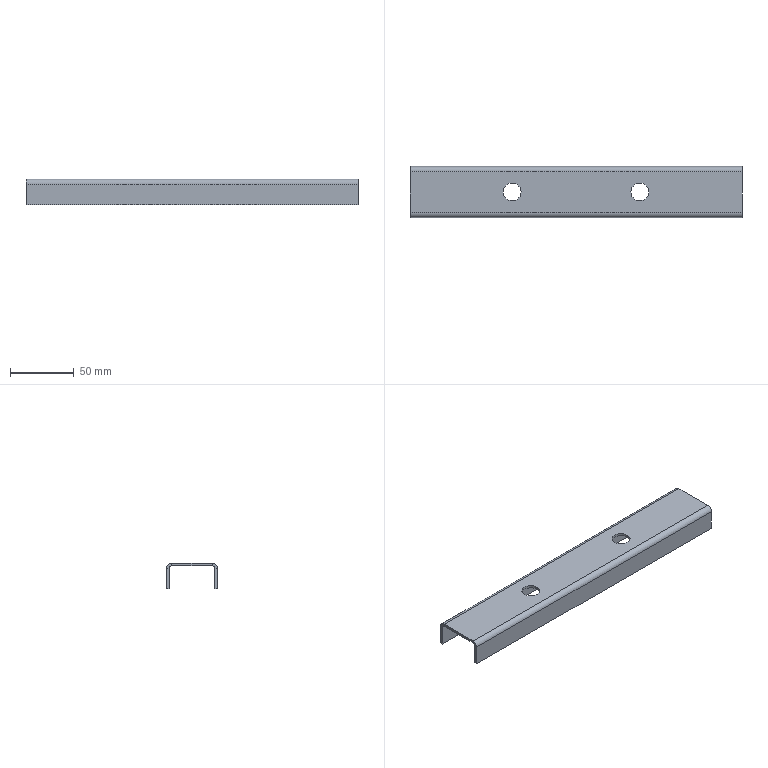Part | STEP file | Produce dryer line heating fan-OVEN-454 | 1 solid | 26 faces | box 260 x 40 x 20 mm | volume 37565 mm3 | plane 18 | cylinder 8 | commonest cylinder face diameters 14 x4 4 x2 8 x2
STEP:
#1=CARTESIAN_POINT('',(57.,20.,-2.));
#2=VERTEX_POINT('',#1);
#3=CARTESIAN_POINT('',(43.,20.,-2.));
#4=VERTEX_POINT('',#3);
#5=CARTESIAN_POINT('',(50.,20.,-2.));
#6=DIRECTION('',(0.,0.,-1.));
#7=DIRECTION('',(-1.,0.,0.));
#8=AXIS2_PLACEMENT_3D('',#5,#6,#7);
#9=CIRCLE('',#8,7.);
#10=EDGE_CURVE('',#2,#4,#9,.T.);
#11=ORIENTED_EDGE('',*,*,#10,.T.);
#12=CARTESIAN_POINT('',(43.,20.,0.));
#13=VERTEX_POINT('',#12);
#14=CARTESIAN_POINT('',(43.,20.,-10.));
#15=DIRECTION('',(0.,0.,1.));
#16=VECTOR('',#15,1000.);
#17=LINE('',#14,#16);
#18=EDGE_CURVE('',#4,#13,#17,.T.);
#19=ORIENTED_EDGE('',*,*,#18,.T.);
#20=CARTESIAN_POINT('',(57.,20.,0.));
#21=VERTEX_POINT('',#20);
#22=CARTESIAN_POINT('',(50.,20.,0.));
#23=DIRECTION('',(0.,0.,1.));
#24=DIRECTION('',(1.,0.,0.));
#25=AXIS2_PLACEMENT_3D('',#22,#23,#24);
#26=CIRCLE('',#25,7.);
#27=EDGE_CURVE('',#13,#21,#26,.T.);
#28=ORIENTED_EDGE('',*,*,#27,.T.);
#29=CARTESIAN_POINT('',(57.,20.,-10.));
#30=DIRECTION('',(0.,0.,1.));
#31=VECTOR('',#30,1000.);
#32=LINE('',#29,#31);
#33=EDGE_CURVE('',#2,#21,#32,.T.);
#34=ORIENTED_EDGE('',*,*,#33,.F.);
#35=EDGE_LOOP('',(#11,#19,#28,#34));
#36=FACE_OUTER_BOUND('',#35,.T.);
#37=CARTESIAN_POINT('',(50.,20.,-10.));
#38=DIRECTION('',(0.,0.,1.));
#39=DIRECTION('',(1.,0.,0.));
#40=AXIS2_PLACEMENT_3D('',#37,#38,#39);
#41=CYLINDRICAL_SURFACE('',#40,7.);
#42=ADVANCED_FACE('',(#36),#41,.F.);
#43=CARTESIAN_POINT('',(-43.,20.,-2.));
#44=VERTEX_POINT('',#43);
#45=CARTESIAN_POINT('',(-57.,20.,-2.));
#46=VERTEX_POINT('',#45);
#47=CARTESIAN_POINT('',(-50.,20.,-2.));
#48=DIRECTION('',(0.,0.,-1.));
#49=DIRECTION('',(-1.,0.,0.));
#50=AXIS2_PLACEMENT_3D('',#47,#48,#49);
#51=CIRCLE('',#50,7.);
#52=EDGE_CURVE('',#44,#46,#51,.T.);
#53=ORIENTED_EDGE('',*,*,#52,.T.);
#54=CARTESIAN_POINT('',(-57.,20.,0.));
#55=VERTEX_POINT('',#54);
#56=CARTESIAN_POINT('',(-57.,20.,-10.));
#57=DIRECTION('',(0.,0.,1.));
#58=VECTOR('',#57,1000.);
#59=LINE('',#56,#58);
#60=EDGE_CURVE('',#46,#55,#59,.T.);
#61=ORIENTED_EDGE('',*,*,#60,.T.);
#62=CARTESIAN_POINT('',(-43.,20.,0.));
#63=VERTEX_POINT('',#62);
#64=CARTESIAN_POINT('',(-50.,20.,0.));
#65=DIRECTION('',(0.,0.,1.));
#66=DIRECTION('',(1.,0.,0.));
#67=AXIS2_PLACEMENT_3D('',#64,#65,#66);
#68=CIRCLE('',#67,7.);
#69=EDGE_CURVE('',#55,#63,#68,.T.);
#70=ORIENTED_EDGE('',*,*,#69,.T.);
#71=CARTESIAN_POINT('',(-43.,20.,-10.));
#72=DIRECTION('',(0.,0.,1.));
#73=VECTOR('',#72,1000.);
#74=LINE('',#71,#73);
#75=EDGE_CURVE('',#44,#63,#74,.T.);
#76=ORIENTED_EDGE('',*,*,#75,.F.);
#77=EDGE_LOOP('',(#53,#61,#70,#76));
#78=FACE_OUTER_BOUND('',#77,.T.);
#79=CARTESIAN_POINT('',(-50.,20.,-10.));
#80=DIRECTION('',(0.,0.,1.));
#81=DIRECTION('',(1.,0.,0.));
#82=AXIS2_PLACEMENT_3D('',#79,#80,#81);
#83=CYLINDRICAL_SURFACE('',#82,7.);
#84=ADVANCED_FACE('',(#78),#83,.F.);
#85=CARTESIAN_POINT('',(130.,4.,0.));
#86=VERTEX_POINT('',#85);
#87=CARTESIAN_POINT('',(130.,4.,-2.));
#88=VERTEX_POINT('',#87);
#89=CARTESIAN_POINT('',(130.,4.,0.));
#90=DIRECTION('',(0.,0.,-1.));
#91=VECTOR('',#90,1000.);
#92=LINE('',#89,#91);
#93=EDGE_CURVE('',#86,#88,#92,.T.);
#94=ORIENTED_EDGE('',*,*,#93,.F.);
#95=CARTESIAN_POINT('',(130.,0.,-4.));
#96=VERTEX_POINT('',#95);
#97=CARTESIAN_POINT('',(130.,4.,-4.));
#98=DIRECTION('',(1.,0.,0.));
#99=DIRECTION('',(0.,0.,-1.));
#100=AXIS2_PLACEMENT_3D('',#97,#98,#99);
#101=CIRCLE('',#100,4.);
#102=EDGE_CURVE('',#86,#96,#101,.T.);
#103=ORIENTED_EDGE('',*,*,#102,.T.);
#104=CARTESIAN_POINT('',(130.,2.,-4.));
#105=VERTEX_POINT('',#104);
#106=CARTESIAN_POINT('',(130.,2.,-4.));
#107=DIRECTION('',(0.,-1.,0.));
#108=VECTOR('',#107,1000.);
#109=LINE('',#106,#108);
#110=EDGE_CURVE('',#105,#96,#109,.T.);
#111=ORIENTED_EDGE('',*,*,#110,.F.);
#112=CARTESIAN_POINT('',(130.,4.,-4.));
#113=DIRECTION('',(1.,0.,0.));
#114=DIRECTION('',(0.,0.,-1.));
#115=AXIS2_PLACEMENT_3D('',#112,#113,#114);
#116=CIRCLE('',#115,2.);
#117=EDGE_CURVE('',#88,#105,#116,.T.);
#118=ORIENTED_EDGE('',*,*,#117,.F.);
#119=EDGE_LOOP('',(#94,#103,#111,#118));
#120=FACE_OUTER_BOUND('',#119,.T.);
#121=CARTESIAN_POINT('',(130.,4.,0.));
#122=DIRECTION('',(1.,0.,0.));
#123=DIRECTION('',(0.,0.,-1.));
#124=AXIS2_PLACEMENT_3D('',#121,#122,#123);
#125=PLANE('',#124);
#126=ADVANCED_FACE('',(#120),#125,.T.);
#127=CARTESIAN_POINT('',(130.,36.,0.));
#128=VERTEX_POINT('',#127);
#129=CARTESIAN_POINT('',(130.,40.,0.));
#130=DIRECTION('',(0.,-1.,0.));
#131=VECTOR('',#130,1000.);
#132=LINE('',#129,#131);
#133=EDGE_CURVE('',#128,#86,#132,.T.);
#134=ORIENTED_EDGE('',*,*,#133,.T.);
#135=ORIENTED_EDGE('',*,*,#93,.T.);
#136=CARTESIAN_POINT('',(130.,36.,-2.));
#137=VERTEX_POINT('',#136);
#138=CARTESIAN_POINT('',(130.,40.,-2.));
#139=DIRECTION('',(0.,-1.,0.));
#140=VECTOR('',#139,1000.);
#141=LINE('',#138,#140);
#142=EDGE_CURVE('',#137,#88,#141,.T.);
#143=ORIENTED_EDGE('',*,*,#142,.F.);
#144=CARTESIAN_POINT('',(130.,36.,-2.));
#145=DIRECTION('',(0.,0.,1.));
#146=VECTOR('',#145,1000.);
#147=LINE('',#144,#146);
#148=EDGE_CURVE('',#137,#128,#147,.T.);
#149=ORIENTED_EDGE('',*,*,#148,.T.);
#150=EDGE_LOOP('',(#134,#135,#143,#149));
#151=FACE_OUTER_BOUND('',#150,.T.);
#152=CARTESIAN_POINT('',(130.,2.,-4.));
#153=DIRECTION('',(1.,0.,0.));
#154=DIRECTION('',(0.,0.,-1.));
#155=AXIS2_PLACEMENT_3D('',#152,#153,#154);
#156=PLANE('',#155);
#157=ADVANCED_FACE('',(#151),#156,.T.);
#158=CARTESIAN_POINT('',(-130.,0.,-4.));
#159=VERTEX_POINT('',#158);
#160=CARTESIAN_POINT('',(-130.,2.,-4.));
#161=VERTEX_POINT('',#160);
#162=CARTESIAN_POINT('',(-130.,0.,-4.));
#163=DIRECTION('',(0.,1.,0.));
#164=VECTOR('',#163,1000.);
#165=LINE('',#162,#164);
#166=EDGE_CURVE('',#159,#161,#165,.T.);
#167=ORIENTED_EDGE('',*,*,#166,.F.);
#168=CARTESIAN_POINT('',(-130.,4.,0.));
#169=VERTEX_POINT('',#168);
#170=CARTESIAN_POINT('',(-130.,4.,-4.));
#171=DIRECTION('',(1.,0.,0.));
#172=DIRECTION('',(0.,0.,-1.));
#173=AXIS2_PLACEMENT_3D('',#170,#171,#172);
#174=CIRCLE('',#173,4.);
#175=EDGE_CURVE('',#169,#159,#174,.T.);
#176=ORIENTED_EDGE('',*,*,#175,.F.);
#177=CARTESIAN_POINT('',(-130.,4.,-2.));
#178=VERTEX_POINT('',#177);
#179=CARTESIAN_POINT('',(-130.,4.,-2.));
#180=DIRECTION('',(0.,0.,1.));
#181=VECTOR('',#180,1000.);
#182=LINE('',#179,#181);
#183=EDGE_CURVE('',#178,#169,#182,.T.);
#184=ORIENTED_EDGE('',*,*,#183,.F.);
#185=CARTESIAN_POINT('',(-130.,4.,-4.));
#186=DIRECTION('',(1.,0.,0.));
#187=DIRECTION('',(0.,0.,-1.));
#188=AXIS2_PLACEMENT_3D('',#185,#186,#187);
#189=CIRCLE('',#188,2.);
#190=EDGE_CURVE('',#178,#161,#189,.T.);
#191=ORIENTED_EDGE('',*,*,#190,.T.);
#192=EDGE_LOOP('',(#167,#176,#184,#191));
#193=FACE_OUTER_BOUND('',#192,.T.);
#194=CARTESIAN_POINT('',(-130.,0.,-4.));
#195=DIRECTION('',(-1.,0.,0.));
#196=DIRECTION('',(0.,0.,1.));
#197=AXIS2_PLACEMENT_3D('',#194,#195,#196);
#198=PLANE('',#197);
#199=ADVANCED_FACE('',(#193),#198,.T.);
#200=CARTESIAN_POINT('',(-130.,0.,-20.));
#201=VERTEX_POINT('',#200);
#202=CARTESIAN_POINT('',(-130.,0.,0.));
#203=DIRECTION('',(0.,0.,-1.));
#204=VECTOR('',#203,1000.);
#205=LINE('',#202,#204);
#206=EDGE_CURVE('',#159,#201,#205,.T.);
#207=ORIENTED_EDGE('',*,*,#206,.F.);
#208=ORIENTED_EDGE('',*,*,#166,.T.);
#209=CARTESIAN_POINT('',(-130.,2.,-20.));
#210=VERTEX_POINT('',#209);
#211=CARTESIAN_POINT('',(-130.,2.,0.));
#212=DIRECTION('',(0.,0.,-1.));
#213=VECTOR('',#212,1000.);
#214=LINE('',#211,#213);
#215=EDGE_CURVE('',#161,#210,#214,.T.);
#216=ORIENTED_EDGE('',*,*,#215,.T.);
#217=CARTESIAN_POINT('',(-130.,2.,-20.));
#218=DIRECTION('',(0.,-1.,0.));
#219=VECTOR('',#218,1000.);
#220=LINE('',#217,#219);
#221=EDGE_CURVE('',#210,#201,#220,.T.);
#222=ORIENTED_EDGE('',*,*,#221,.T.);
#223=EDGE_LOOP('',(#207,#208,#216,#222));
#224=FACE_OUTER_BOUND('',#223,.T.);
#225=CARTESIAN_POINT('',(-130.,4.,-2.));
#226=DIRECTION('',(-1.,0.,0.));
#227=DIRECTION('',(0.,0.,1.));
#228=AXIS2_PLACEMENT_3D('',#225,#226,#227);
#229=PLANE('',#228);
#230=ADVANCED_FACE('',(#224),#229,.T.);
#231=CARTESIAN_POINT('',(130.,40.,-4.));
#232=VERTEX_POINT('',#231);
#233=CARTESIAN_POINT('',(130.,38.,-4.));
#234=VERTEX_POINT('',#233);
#235=CARTESIAN_POINT('',(130.,40.,-4.));
#236=DIRECTION('',(0.,-1.,0.));
#237=VECTOR('',#236,1000.);
#238=LINE('',#235,#237);
#239=EDGE_CURVE('',#232,#234,#238,.T.);
#240=ORIENTED_EDGE('',*,*,#239,.F.);
#241=CARTESIAN_POINT('',(130.,36.,-4.));
#242=DIRECTION('',(1.,0.,0.));
#243=DIRECTION('',(0.,0.,-1.));
#244=AXIS2_PLACEMENT_3D('',#241,#242,#243);
#245=CIRCLE('',#244,4.);
#246=EDGE_CURVE('',#232,#128,#245,.T.);
#247=ORIENTED_EDGE('',*,*,#246,.T.);
#248=ORIENTED_EDGE('',*,*,#148,.F.);
#249=CARTESIAN_POINT('',(130.,36.,-4.));
#250=DIRECTION('',(1.,0.,0.));
#251=DIRECTION('',(0.,0.,-1.));
#252=AXIS2_PLACEMENT_3D('',#249,#250,#251);
#253=CIRCLE('',#252,2.);
#254=EDGE_CURVE('',#234,#137,#253,.T.);
#255=ORIENTED_EDGE('',*,*,#254,.F.);
#256=EDGE_LOOP('',(#240,#247,#248,#255));
#257=FACE_OUTER_BOUND('',#256,.T.);
#258=CARTESIAN_POINT('',(130.,40.,-4.));
#259=DIRECTION('',(1.,0.,0.));
#260=DIRECTION('',(0.,0.,-1.));
#261=AXIS2_PLACEMENT_3D('',#258,#259,#260);
#262=PLANE('',#261);
#263=ADVANCED_FACE('',(#257),#262,.T.);
#264=CARTESIAN_POINT('',(130.,40.,-20.));
#265=VERTEX_POINT('',#264);
#266=CARTESIAN_POINT('',(130.,40.,0.));
#267=DIRECTION('',(0.,0.,1.));
#268=VECTOR('',#267,1000.);
#269=LINE('',#266,#268);
#270=EDGE_CURVE('',#265,#232,#269,.T.);
#271=ORIENTED_EDGE('',*,*,#270,.T.);
#272=ORIENTED_EDGE('',*,*,#239,.T.);
#273=CARTESIAN_POINT('',(130.,38.,-20.));
#274=VERTEX_POINT('',#273);
#275=CARTESIAN_POINT('',(130.,38.,0.));
#276=DIRECTION('',(0.,0.,1.));
#277=VECTOR('',#276,1000.);
#278=LINE('',#275,#277);
#279=EDGE_CURVE('',#274,#234,#278,.T.);
#280=ORIENTED_EDGE('',*,*,#279,.F.);
#281=CARTESIAN_POINT('',(130.,40.,-20.));
#282=DIRECTION('',(0.,-1.,0.));
#283=VECTOR('',#282,1000.);
#284=LINE('',#281,#283);
#285=EDGE_CURVE('',#265,#274,#284,.T.);
#286=ORIENTED_EDGE('',*,*,#285,.F.);
#287=EDGE_LOOP('',(#271,#272,#280,#286));
#288=FACE_OUTER_BOUND('',#287,.T.);
#289=CARTESIAN_POINT('',(130.,36.,-2.));
#290=DIRECTION('',(1.,0.,0.));
#291=DIRECTION('',(0.,0.,-1.));
#292=AXIS2_PLACEMENT_3D('',#289,#290,#291);
#293=PLANE('',#292);
#294=ADVANCED_FACE('',(#288),#293,.T.);
#295=CARTESIAN_POINT('',(-130.,36.,0.));
#296=VERTEX_POINT('',#295);
#297=CARTESIAN_POINT('',(-130.,36.,-2.));
#298=VERTEX_POINT('',#297);
#299=CARTESIAN_POINT('',(-130.,36.,0.));
#300=DIRECTION('',(0.,0.,-1.));
#301=VECTOR('',#300,1000.);
#302=LINE('',#299,#301);
#303=EDGE_CURVE('',#296,#298,#302,.T.);
#304=ORIENTED_EDGE('',*,*,#303,.F.);
#305=CARTESIAN_POINT('',(-130.,40.,-4.));
#306=VERTEX_POINT('',#305);
#307=CARTESIAN_POINT('',(-130.,36.,-4.));
#308=DIRECTION('',(1.,0.,0.));
#309=DIRECTION('',(0.,0.,-1.));
#310=AXIS2_PLACEMENT_3D('',#307,#308,#309);
#311=CIRCLE('',#310,4.);
#312=EDGE_CURVE('',#306,#296,#311,.T.);
#313=ORIENTED_EDGE('',*,*,#312,.F.);
#314=CARTESIAN_POINT('',(-130.,38.,-4.));
#315=VERTEX_POINT('',#314);
#316=CARTESIAN_POINT('',(-130.,38.,-4.));
#317=DIRECTION('',(0.,1.,0.));
#318=VECTOR('',#317,1000.);
#319=LINE('',#316,#318);
#320=EDGE_CURVE('',#315,#306,#319,.T.);
#321=ORIENTED_EDGE('',*,*,#320,.F.);
#322=CARTESIAN_POINT('',(-130.,36.,-4.));
#323=DIRECTION('',(1.,0.,0.));
#324=DIRECTION('',(0.,0.,-1.));
#325=AXIS2_PLACEMENT_3D('',#322,#323,#324);
#326=CIRCLE('',#325,2.);
#327=EDGE_CURVE('',#315,#298,#326,.T.);
#328=ORIENTED_EDGE('',*,*,#327,.T.);
#329=EDGE_LOOP('',(#304,#313,#321,#328));
#330=FACE_OUTER_BOUND('',#329,.T.);
#331=CARTESIAN_POINT('',(-130.,36.,0.));
#332=DIRECTION('',(-1.,0.,0.));
#333=DIRECTION('',(0.,0.,1.));
#334=AXIS2_PLACEMENT_3D('',#331,#332,#333);
#335=PLANE('',#334);
#336=ADVANCED_FACE('',(#330),#335,.T.);
#337=CARTESIAN_POINT('',(-130.,40.,0.));
#338=DIRECTION('',(0.,-1.,0.));
#339=VECTOR('',#338,1000.);
#340=LINE('',#337,#339);
#341=EDGE_CURVE('',#296,#169,#340,.T.);
#342=ORIENTED_EDGE('',*,*,#341,.F.);
#343=ORIENTED_EDGE('',*,*,#303,.T.);
#344=CARTESIAN_POINT('',(-130.,40.,-2.));
#345=DIRECTION('',(0.,-1.,0.));
#346=VECTOR('',#345,1000.);
#347=LINE('',#344,#346);
#348=EDGE_CURVE('',#298,#178,#347,.T.);
#349=ORIENTED_EDGE('',*,*,#348,.T.);
#350=ORIENTED_EDGE('',*,*,#183,.T.);
#351=EDGE_LOOP('',(#342,#343,#349,#350));
#352=FACE_OUTER_BOUND('',#351,.T.);
#353=CARTESIAN_POINT('',(-130.,38.,-4.));
#354=DIRECTION('',(-1.,0.,0.));
#355=DIRECTION('',(0.,0.,1.));
#356=AXIS2_PLACEMENT_3D('',#353,#354,#355);
#357=PLANE('',#356);
#358=ADVANCED_FACE('',(#352),#357,.T.);
#359=ORIENTED_EDGE('',*,*,#206,.T.);
#360=CARTESIAN_POINT('',(130.,0.,-20.));
#361=VERTEX_POINT('',#360);
#362=CARTESIAN_POINT('',(130.,0.,-20.));
#363=DIRECTION('',(-1.,0.,0.));
#364=VECTOR('',#363,1000.);
#365=LINE('',#362,#364);
#366=EDGE_CURVE('',#361,#201,#365,.T.);
#367=ORIENTED_EDGE('',*,*,#366,.F.);
#368=CARTESIAN_POINT('',(130.,0.,0.));
#369=DIRECTION('',(0.,0.,-1.));
#370=VECTOR('',#369,1000.);
#371=LINE('',#368,#370);
#372=EDGE_CURVE('',#96,#361,#371,.T.);
#373=ORIENTED_EDGE('',*,*,#372,.F.);
#374=CARTESIAN_POINT('',(130.,0.,-4.));
#375=DIRECTION('',(-1.,0.,0.));
#376=VECTOR('',#375,1000.);
#377=LINE('',#374,#376);
#378=EDGE_CURVE('',#96,#159,#377,.T.);
#379=ORIENTED_EDGE('',*,*,#378,.T.);
#380=EDGE_LOOP('',(#359,#367,#373,#379));
#381=FACE_OUTER_BOUND('',#380,.T.);
#382=CARTESIAN_POINT('',(130.,0.,0.));
#383=DIRECTION('',(0.,1.,0.));
#384=DIRECTION('',(0.,0.,1.));
#385=AXIS2_PLACEMENT_3D('',#382,#383,#384);
#386=PLANE('',#385);
#387=ADVANCED_FACE('',(#381),#386,.F.);
#388=ORIENTED_EDGE('',*,*,#221,.F.);
#389=CARTESIAN_POINT('',(130.,2.,-20.));
#390=VERTEX_POINT('',#389);
#391=CARTESIAN_POINT('',(130.,2.,-20.));
#392=DIRECTION('',(-1.,0.,0.));
#393=VECTOR('',#392,1000.);
#394=LINE('',#391,#393);
#395=EDGE_CURVE('',#390,#210,#394,.T.);
#396=ORIENTED_EDGE('',*,*,#395,.F.);
#397=CARTESIAN_POINT('',(130.,2.,-20.));
#398=DIRECTION('',(0.,-1.,0.));
#399=VECTOR('',#398,1000.);
#400=LINE('',#397,#399);
#401=EDGE_CURVE('',#390,#361,#400,.T.);
#402=ORIENTED_EDGE('',*,*,#401,.T.);
#403=ORIENTED_EDGE('',*,*,#366,.T.);
#404=EDGE_LOOP('',(#388,#396,#402,#403));
#405=FACE_OUTER_BOUND('',#404,.T.);
#406=CARTESIAN_POINT('',(130.,2.,-20.));
#407=DIRECTION('',(0.,0.,-1.));
#408=DIRECTION('',(-1.,0.,0.));
#409=AXIS2_PLACEMENT_3D('',#406,#407,#408);
#410=PLANE('',#409);
#411=ADVANCED_FACE('',(#405),#410,.T.);
#412=ORIENTED_EDGE('',*,*,#215,.F.);
#413=CARTESIAN_POINT('',(130.,2.,-4.));
#414=DIRECTION('',(-1.,0.,0.));
#415=VECTOR('',#414,1000.);
#416=LINE('',#413,#415);
#417=EDGE_CURVE('',#105,#161,#416,.T.);
#418=ORIENTED_EDGE('',*,*,#417,.F.);
#419=CARTESIAN_POINT('',(130.,2.,0.));
#420=DIRECTION('',(0.,0.,-1.));
#421=VECTOR('',#420,1000.);
#422=LINE('',#419,#421);
#423=EDGE_CURVE('',#105,#390,#422,.T.);
#424=ORIENTED_EDGE('',*,*,#423,.T.);
#425=ORIENTED_EDGE('',*,*,#395,.T.);
#426=EDGE_LOOP('',(#412,#418,#424,#425));
#427=FACE_OUTER_BOUND('',#426,.T.);
#428=CARTESIAN_POINT('',(130.,2.,0.));
#429=DIRECTION('',(0.,1.,0.));
#430=DIRECTION('',(0.,0.,1.));
#431=AXIS2_PLACEMENT_3D('',#428,#429,#430);
#432=PLANE('',#431);
#433=ADVANCED_FACE('',(#427),#432,.T.);
#434=ORIENTED_EDGE('',*,*,#190,.F.);
#435=CARTESIAN_POINT('',(130.,4.,-2.));
#436=DIRECTION('',(-1.,0.,0.));
#437=VECTOR('',#436,1000.);
#438=LINE('',#435,#437);
#439=EDGE_CURVE('',#88,#178,#438,.T.);
#440=ORIENTED_EDGE('',*,*,#439,.F.);
#441=ORIENTED_EDGE('',*,*,#117,.T.);
#442=ORIENTED_EDGE('',*,*,#417,.T.);
#443=EDGE_LOOP('',(#434,#440,#441,#442));
#444=FACE_OUTER_BOUND('',#443,.T.);
#445=CARTESIAN_POINT('',(130.,4.,-4.));
#446=DIRECTION('',(-1.,0.,0.));
#447=DIRECTION('',(0.,0.,1.));
#448=AXIS2_PLACEMENT_3D('',#445,#446,#447);
#449=CYLINDRICAL_SURFACE('',#448,2.);
#450=ADVANCED_FACE('',(#444),#449,.F.);
#451=ORIENTED_EDGE('',*,*,#10,.F.);
#452=CARTESIAN_POINT('',(50.,20.,-2.));
#453=DIRECTION('',(0.,0.,-1.));
#454=DIRECTION('',(-1.,0.,0.));
#455=AXIS2_PLACEMENT_3D('',#452,#453,#454);
#456=CIRCLE('',#455,7.);
#457=EDGE_CURVE('',#4,#2,#456,.T.);
#458=ORIENTED_EDGE('',*,*,#457,.F.);
#459=EDGE_LOOP('',(#451,#458));
#460=FACE_BOUND('',#459,.T.);
#461=ORIENTED_EDGE('',*,*,#52,.F.);
#462=CARTESIAN_POINT('',(-50.,20.,-2.));
#463=DIRECTION('',(0.,0.,-1.));
#464=DIRECTION('',(-1.,0.,0.));
#465=AXIS2_PLACEMENT_3D('',#462,#463,#464);
#466=CIRCLE('',#465,7.);
#467=EDGE_CURVE('',#46,#44,#466,.T.);
#468=ORIENTED_EDGE('',*,*,#467,.F.);
#469=EDGE_LOOP('',(#461,#468));
#470=FACE_BOUND('',#469,.T.);
#471=ORIENTED_EDGE('',*,*,#348,.F.);
#472=CARTESIAN_POINT('',(130.,36.,-2.));
#473=DIRECTION('',(-1.,0.,0.));
#474=VECTOR('',#473,1000.);
#475=LINE('',#472,#474);
#476=EDGE_CURVE('',#137,#298,#475,.T.);
#477=ORIENTED_EDGE('',*,*,#476,.F.);
#478=ORIENTED_EDGE('',*,*,#142,.T.);
#479=ORIENTED_EDGE('',*,*,#439,.T.);
#480=EDGE_LOOP('',(#471,#477,#478,#479));
#481=FACE_OUTER_BOUND('',#480,.T.);
#482=CARTESIAN_POINT('',(130.,40.,-2.));
#483=DIRECTION('',(0.,0.,-1.));
#484=DIRECTION('',(-1.,0.,0.));
#485=AXIS2_PLACEMENT_3D('',#482,#483,#484);
#486=PLANE('',#485);
#487=ADVANCED_FACE('',(#460,#470,#481),#486,.T.);
#488=ORIENTED_EDGE('',*,*,#327,.F.);
#489=CARTESIAN_POINT('',(130.,38.,-4.));
#490=DIRECTION('',(-1.,0.,0.));
#491=VECTOR('',#490,1000.);
#492=LINE('',#489,#491);
#493=EDGE_CURVE('',#234,#315,#492,.T.);
#494=ORIENTED_EDGE('',*,*,#493,.F.);
#495=ORIENTED_EDGE('',*,*,#254,.T.);
#496=ORIENTED_EDGE('',*,*,#476,.T.);
#497=EDGE_LOOP('',(#488,#494,#495,#496));
#498=FACE_OUTER_BOUND('',#497,.T.);
#499=CARTESIAN_POINT('',(130.,36.,-4.));
#500=DIRECTION('',(-1.,0.,0.));
#501=DIRECTION('',(0.,0.,1.));
#502=AXIS2_PLACEMENT_3D('',#499,#500,#501);
#503=CYLINDRICAL_SURFACE('',#502,2.);
#504=ADVANCED_FACE('',(#498),#503,.F.);
#505=CARTESIAN_POINT('',(-130.,38.,-20.));
#506=VERTEX_POINT('',#505);
#507=CARTESIAN_POINT('',(-130.,38.,0.));
#508=DIRECTION('',(0.,0.,1.));
#509=VECTOR('',#508,1000.);
#510=LINE('',#507,#509);
#511=EDGE_CURVE('',#506,#315,#510,.T.);
#512=ORIENTED_EDGE('',*,*,#511,.F.);
#513=CARTESIAN_POINT('',(130.,38.,-20.));
#514=DIRECTION('',(-1.,0.,0.));
#515=VECTOR('',#514,1000.);
#516=LINE('',#513,#515);
#517=EDGE_CURVE('',#274,#506,#516,.T.);
#518=ORIENTED_EDGE('',*,*,#517,.F.);
#519=ORIENTED_EDGE('',*,*,#279,.T.);
#520=ORIENTED_EDGE('',*,*,#493,.T.);
#521=EDGE_LOOP('',(#512,#518,#519,#520));
#522=FACE_OUTER_BOUND('',#521,.T.);
#523=CARTESIAN_POINT('',(130.,38.,0.));
#524=DIRECTION('',(0.,-1.,0.));
#525=DIRECTION('',(0.,0.,-1.));
#526=AXIS2_PLACEMENT_3D('',#523,#524,#525);
#527=PLANE('',#526);
#528=ADVANCED_FACE('',(#522),#527,.T.);
#529=CARTESIAN_POINT('',(-130.,40.,-20.));
#530=VERTEX_POINT('',#529);
#531=CARTESIAN_POINT('',(-130.,40.,-20.));
#532=DIRECTION('',(0.,-1.,0.));
#533=VECTOR('',#532,1000.);
#534=LINE('',#531,#533);
#535=EDGE_CURVE('',#530,#506,#534,.T.);
#536=ORIENTED_EDGE('',*,*,#535,.F.);
#537=CARTESIAN_POINT('',(130.,40.,-20.));
#538=DIRECTION('',(-1.,0.,0.));
#539=VECTOR('',#538,1000.);
#540=LINE('',#537,#539);
#541=EDGE_CURVE('',#265,#530,#540,.T.);
#542=ORIENTED_EDGE('',*,*,#541,.F.);
#543=ORIENTED_EDGE('',*,*,#285,.T.);
#544=ORIENTED_EDGE('',*,*,#517,.T.);
#545=EDGE_LOOP('',(#536,#542,#543,#544));
#546=FACE_OUTER_BOUND('',#545,.T.);
#547=CARTESIAN_POINT('',(130.,40.,-20.));
#548=DIRECTION('',(0.,0.,-1.));
#549=DIRECTION('',(-1.,0.,0.));
#550=AXIS2_PLACEMENT_3D('',#547,#548,#549);
#551=PLANE('',#550);
#552=ADVANCED_FACE('',(#546),#551,.T.);
#553=CARTESIAN_POINT('',(-130.,40.,0.));
#554=DIRECTION('',(0.,0.,1.));
#555=VECTOR('',#554,1000.);
#556=LINE('',#553,#555);
#557=EDGE_CURVE('',#530,#306,#556,.T.);
#558=ORIENTED_EDGE('',*,*,#557,.T.);
#559=CARTESIAN_POINT('',(130.,40.,-4.));
#560=DIRECTION('',(-1.,0.,0.));
#561=VECTOR('',#560,1000.);
#562=LINE('',#559,#561);
#563=EDGE_CURVE('',#232,#306,#562,.T.);
#564=ORIENTED_EDGE('',*,*,#563,.F.);
#565=ORIENTED_EDGE('',*,*,#270,.F.);
#566=ORIENTED_EDGE('',*,*,#541,.T.);
#567=EDGE_LOOP('',(#558,#564,#565,#566));
#568=FACE_OUTER_BOUND('',#567,.T.);
#569=CARTESIAN_POINT('',(130.,40.,0.));
#570=DIRECTION('',(0.,-1.,0.));
#571=DIRECTION('',(0.,0.,-1.));
#572=AXIS2_PLACEMENT_3D('',#569,#570,#571);
#573=PLANE('',#572);
#574=ADVANCED_FACE('',(#568),#573,.F.);
#575=ORIENTED_EDGE('',*,*,#312,.T.);
#576=CARTESIAN_POINT('',(130.,36.,0.));
#577=DIRECTION('',(-1.,0.,0.));
#578=VECTOR('',#577,1000.);
#579=LINE('',#576,#578);
#580=EDGE_CURVE('',#128,#296,#579,.T.);
#581=ORIENTED_EDGE('',*,*,#580,.F.);
#582=ORIENTED_EDGE('',*,*,#246,.F.);
#583=ORIENTED_EDGE('',*,*,#563,.T.);
#584=EDGE_LOOP('',(#575,#581,#582,#583));
#585=FACE_OUTER_BOUND('',#584,.T.);
#586=CARTESIAN_POINT('',(130.,36.,-4.));
#587=DIRECTION('',(-1.,0.,0.));
#588=DIRECTION('',(0.,0.,1.));
#589=AXIS2_PLACEMENT_3D('',#586,#587,#588);
#590=CYLINDRICAL_SURFACE('',#589,4.);
#591=ADVANCED_FACE('',(#585),#590,.T.);
#592=CARTESIAN_POINT('',(50.,20.,0.));
#593=DIRECTION('',(0.,0.,1.));
#594=DIRECTION('',(1.,0.,0.));
#595=AXIS2_PLACEMENT_3D('',#592,#593,#594);
#596=CIRCLE('',#595,7.);
#597=EDGE_CURVE('',#21,#13,#596,.T.);
#598=ORIENTED_EDGE('',*,*,#597,.F.);
#599=ORIENTED_EDGE('',*,*,#27,.F.);
#600=EDGE_LOOP('',(#598,#599));
#601=FACE_BOUND('',#600,.T.);
#602=CARTESIAN_POINT('',(-50.,20.,0.));
#603=DIRECTION('',(0.,0.,1.));
#604=DIRECTION('',(1.,0.,0.));
#605=AXIS2_PLACEMENT_3D('',#602,#603,#604);
#606=CIRCLE('',#605,7.);
#607=EDGE_CURVE('',#63,#55,#606,.T.);
#608=ORIENTED_EDGE('',*,*,#607,.F.);
#609=ORIENTED_EDGE('',*,*,#69,.F.);
#610=EDGE_LOOP('',(#608,#609));
#611=FACE_BOUND('',#610,.T.);
#612=ORIENTED_EDGE('',*,*,#341,.T.);
#613=CARTESIAN_POINT('',(130.,4.,0.));
#614=DIRECTION('',(-1.,0.,0.));
#615=VECTOR('',#614,1000.);
#616=LINE('',#613,#615);
#617=EDGE_CURVE('',#86,#169,#616,.T.);
#618=ORIENTED_EDGE('',*,*,#617,.F.);
#619=ORIENTED_EDGE('',*,*,#133,.F.);
#620=ORIENTED_EDGE('',*,*,#580,.T.);
#621=EDGE_LOOP('',(#612,#618,#619,#620));
#622=FACE_OUTER_BOUND('',#621,.T.);
#623=CARTESIAN_POINT('',(130.,40.,0.));
#624=DIRECTION('',(0.,0.,-1.));
#625=DIRECTION('',(-1.,0.,0.));
#626=AXIS2_PLACEMENT_3D('',#623,#624,#625);
#627=PLANE('',#626);
#628=ADVANCED_FACE('',(#601,#611,#622),#627,.F.);
#629=ORIENTED_EDGE('',*,*,#175,.T.);
#630=ORIENTED_EDGE('',*,*,#378,.F.);
#631=ORIENTED_EDGE('',*,*,#102,.F.);
#632=ORIENTED_EDGE('',*,*,#617,.T.);
#633=EDGE_LOOP('',(#629,#630,#631,#632));
#634=FACE_OUTER_BOUND('',#633,.T.);
#635=CARTESIAN_POINT('',(130.,4.,-4.));
#636=DIRECTION('',(-1.,0.,0.));
#637=DIRECTION('',(0.,0.,1.));
#638=AXIS2_PLACEMENT_3D('',#635,#636,#637);
#639=CYLINDRICAL_SURFACE('',#638,4.);
#640=ADVANCED_FACE('',(#634),#639,.T.);
#641=ORIENTED_EDGE('',*,*,#372,.T.);
#642=ORIENTED_EDGE('',*,*,#401,.F.);
#643=ORIENTED_EDGE('',*,*,#423,.F.);
#644=ORIENTED_EDGE('',*,*,#110,.T.);
#645=EDGE_LOOP('',(#641,#642,#643,#644));
#646=FACE_OUTER_BOUND('',#645,.T.);
#647=CARTESIAN_POINT('',(130.,4.,-4.));
#648=DIRECTION('',(1.,0.,0.));
#649=DIRECTION('',(0.,0.,-1.));
#650=AXIS2_PLACEMENT_3D('',#647,#648,#649);
#651=PLANE('',#650);
#652=ADVANCED_FACE('',(#646),#651,.T.);
#653=ORIENTED_EDGE('',*,*,#511,.T.);
#654=ORIENTED_EDGE('',*,*,#320,.T.);
#655=ORIENTED_EDGE('',*,*,#557,.F.);
#656=ORIENTED_EDGE('',*,*,#535,.T.);
#657=EDGE_LOOP('',(#653,#654,#655,#656));
#658=FACE_OUTER_BOUND('',#657,.T.);
#659=CARTESIAN_POINT('',(-130.,4.,-4.));
#660=DIRECTION('',(1.,0.,0.));
#661=DIRECTION('',(0.,0.,-1.));
#662=AXIS2_PLACEMENT_3D('',#659,#660,#661);
#663=PLANE('',#662);
#664=ADVANCED_FACE('',(#658),#663,.F.);
#665=ORIENTED_EDGE('',*,*,#60,.F.);
#666=ORIENTED_EDGE('',*,*,#467,.T.);
#667=ORIENTED_EDGE('',*,*,#75,.T.);
#668=ORIENTED_EDGE('',*,*,#607,.T.);
#669=EDGE_LOOP('',(#665,#666,#667,#668));
#670=FACE_OUTER_BOUND('',#669,.T.);
#671=CARTESIAN_POINT('',(-50.,20.,-10.));
#672=DIRECTION('',(0.,0.,1.));
#673=DIRECTION('',(1.,0.,0.));
#674=AXIS2_PLACEMENT_3D('',#671,#672,#673);
#675=CYLINDRICAL_SURFACE('',#674,7.);
#676=ADVANCED_FACE('',(#670),#675,.F.);
#677=ORIENTED_EDGE('',*,*,#18,.F.);
#678=ORIENTED_EDGE('',*,*,#457,.T.);
#679=ORIENTED_EDGE('',*,*,#33,.T.);
#680=ORIENTED_EDGE('',*,*,#597,.T.);
#681=EDGE_LOOP('',(#677,#678,#679,#680));
#682=FACE_OUTER_BOUND('',#681,.T.);
#683=CARTESIAN_POINT('',(50.,20.,-10.));
#684=DIRECTION('',(0.,0.,1.));
#685=DIRECTION('',(1.,0.,0.));
#686=AXIS2_PLACEMENT_3D('',#683,#684,#685);
#687=CYLINDRICAL_SURFACE('',#686,7.);
#688=ADVANCED_FACE('',(#682),#687,.F.);
#689=CLOSED_SHELL('',(#42,#84,#126,#157,#199,#230,#263,#294,#336,#358,#387,#411,#433,#450,#487,#504,#528,#552,#574,#591,#628,#640,#652,#664,#676,#688));
#690=MANIFOLD_SOLID_BREP('',#689);
#691=CARTESIAN_POINT('',(0.,0.,0.));
#692=DIRECTION('',(0.,0.,1.));
#693=DIRECTION('',(1.,0.,0.));
#694=AXIS2_PLACEMENT_3D('',#691,#692,#693);
#695=(LENGTH_UNIT()NAMED_UNIT(*)SI_UNIT(.MILLI.,.METRE.));
#696=UNCERTAINTY_MEASURE_WITH_UNIT(LENGTH_MEASURE(0.00001),#695,'','');
#697=(NAMED_UNIT(*)PLANE_ANGLE_UNIT()SI_UNIT($,.RADIAN.));
#698=(NAMED_UNIT(*)SI_UNIT($,.STERADIAN.)SOLID_ANGLE_UNIT());
#699=(GEOMETRIC_REPRESENTATION_CONTEXT(3)GLOBAL_UNCERTAINTY_ASSIGNED_CONTEXT((#696))GLOBAL_UNIT_ASSIGNED_CONTEXT((#695,#697,#698))REPRESENTATION_CONTEXT('',''));
#700=ADVANCED_BREP_SHAPE_REPRESENTATION('',(#690,#694),#699);